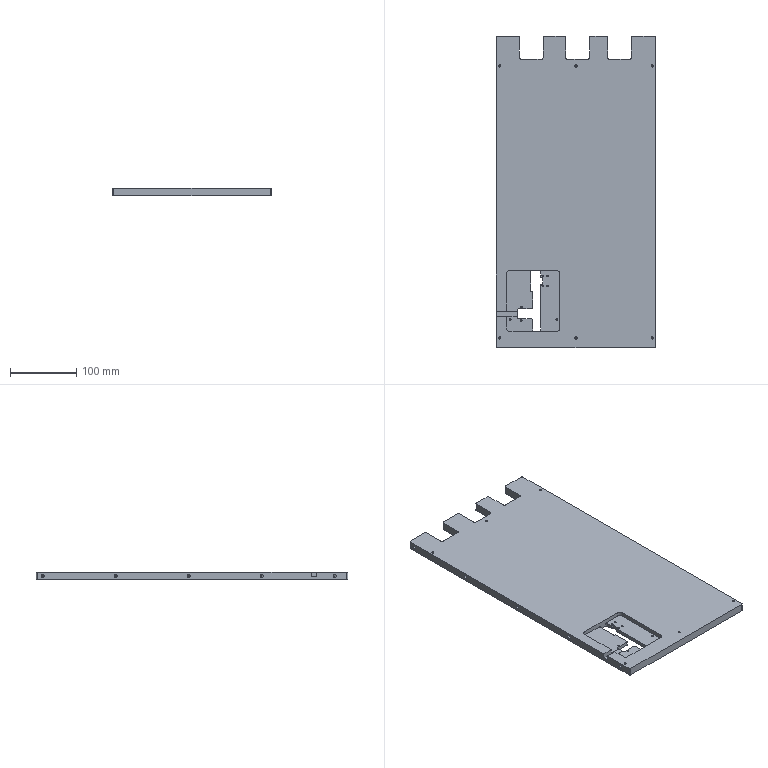Part | NX | features BREP 1 | 1 solid | 244 faces | box 240 x 470 x 12 mm | volume 1246661 mm3 | cylinder 131 | cone 71 | plane 42 | commonest cylinder face diameters 2.5 x78 4 x21 3.3 x12 5 x10 6 x6 10 x4